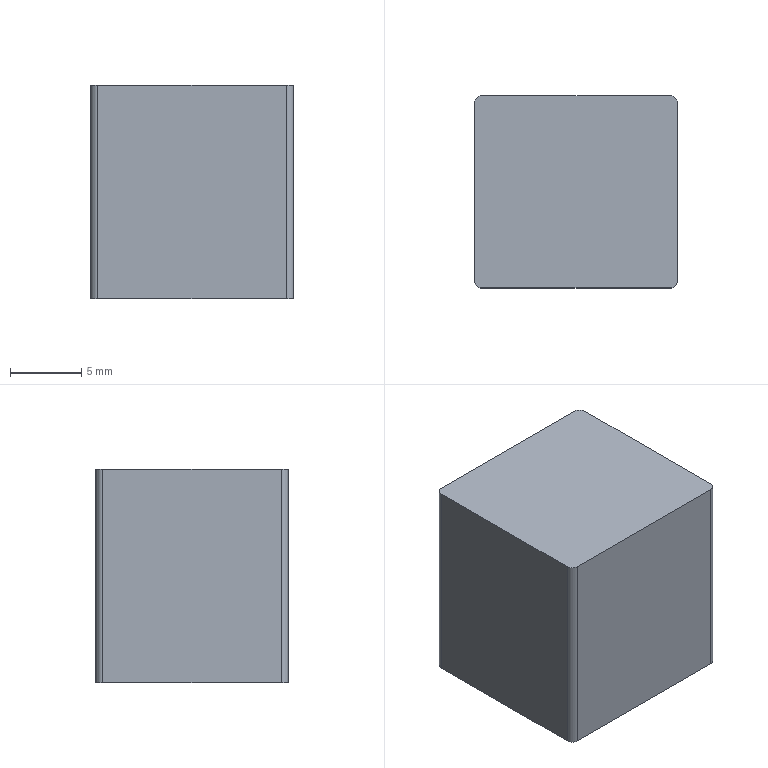Part | NX | features BREP 1 | 1 solid | 10 faces | box 14.274 x 13.522 x 15 mm | volume 2892 mm3 | plane 6 | cylinder 4 | commonest cylinder face diameters 1 x4
STEP:
#1=CARTESIAN_POINT('',(-6.637,6.761,-25.6));
#2=VERTEX_POINT('',#1);
#3=CARTESIAN_POINT('',(-7.137,6.261,-25.6));
#4=VERTEX_POINT('',#3);
#5=CARTESIAN_POINT('',(-6.637,6.261,-25.6));
#6=DIRECTION('',(0.,0.,1.));
#7=DIRECTION('',(1.,0.,0.));
#8=AXIS2_PLACEMENT_3D('',#5,#6,#7);
#9=CIRCLE('',#8,0.5);
#10=EDGE_CURVE('',#2,#4,#9,.T.);
#11=ORIENTED_EDGE('',*,*,#10,.F.);
#12=CARTESIAN_POINT('',(-6.637,6.761,-40.6));
#13=VERTEX_POINT('',#12);
#14=CARTESIAN_POINT('',(-6.637,6.761,-40.6));
#15=DIRECTION('',(0.,0.,1.));
#16=VECTOR('',#15,1000.);
#17=LINE('',#14,#16);
#18=EDGE_CURVE('',#13,#2,#17,.T.);
#19=ORIENTED_EDGE('',*,*,#18,.F.);
#20=CARTESIAN_POINT('',(-7.137,6.261,-40.6));
#21=VERTEX_POINT('',#20);
#22=CARTESIAN_POINT('',(-6.637,6.261,-40.6));
#23=DIRECTION('',(0.,0.,1.));
#24=DIRECTION('',(1.,0.,0.));
#25=AXIS2_PLACEMENT_3D('',#22,#23,#24);
#26=CIRCLE('',#25,0.5);
#27=EDGE_CURVE('',#13,#21,#26,.T.);
#28=ORIENTED_EDGE('',*,*,#27,.T.);
#29=CARTESIAN_POINT('',(-7.137,6.261,-40.6));
#30=DIRECTION('',(0.,0.,1.));
#31=VECTOR('',#30,1000.);
#32=LINE('',#29,#31);
#33=EDGE_CURVE('',#21,#4,#32,.T.);
#34=ORIENTED_EDGE('',*,*,#33,.T.);
#35=EDGE_LOOP('',(#11,#19,#28,#34));
#36=FACE_BOUND('',#35,.T.);
#37=CARTESIAN_POINT('',(-6.637,6.261,-40.6));
#38=DIRECTION('',(0.,0.,1.));
#39=DIRECTION('',(-1.,0.,0.));
#40=AXIS2_PLACEMENT_3D('',#37,#38,#39);
#41=CYLINDRICAL_SURFACE('',#40,0.5);
#42=ADVANCED_FACE('',(#36),#41,.T.);
#43=CARTESIAN_POINT('',(-7.137,-6.261,-25.6));
#44=VERTEX_POINT('',#43);
#45=CARTESIAN_POINT('',(-7.137,-6.261,-25.6));
#46=DIRECTION('',(0.,1.,0.));
#47=VECTOR('',#46,1000.);
#48=LINE('',#45,#47);
#49=EDGE_CURVE('',#44,#4,#48,.T.);
#50=ORIENTED_EDGE('',*,*,#49,.T.);
#51=ORIENTED_EDGE('',*,*,#33,.F.);
#52=CARTESIAN_POINT('',(-7.137,-6.261,-40.6));
#53=VERTEX_POINT('',#52);
#54=CARTESIAN_POINT('',(-7.137,-6.261,-40.6));
#55=DIRECTION('',(0.,1.,0.));
#56=VECTOR('',#55,1000.);
#57=LINE('',#54,#56);
#58=EDGE_CURVE('',#53,#21,#57,.T.);
#59=ORIENTED_EDGE('',*,*,#58,.F.);
#60=CARTESIAN_POINT('',(-7.137,-6.261,-40.6));
#61=DIRECTION('',(0.,0.,1.));
#62=VECTOR('',#61,1000.);
#63=LINE('',#60,#62);
#64=EDGE_CURVE('',#53,#44,#63,.T.);
#65=ORIENTED_EDGE('',*,*,#64,.T.);
#66=EDGE_LOOP('',(#50,#51,#59,#65));
#67=FACE_BOUND('',#66,.T.);
#68=CARTESIAN_POINT('',(-7.137,-6.261,-40.6));
#69=DIRECTION('',(1.,0.,0.));
#70=DIRECTION('',(0.,-1.,0.));
#71=AXIS2_PLACEMENT_3D('',#68,#69,#70);
#72=PLANE('',#71);
#73=ADVANCED_FACE('',(#67),#72,.F.);
#74=CARTESIAN_POINT('',(-6.637,-6.761,-25.6));
#75=VERTEX_POINT('',#74);
#76=CARTESIAN_POINT('',(-6.637,-6.261,-25.6));
#77=DIRECTION('',(0.,0.,1.));
#78=DIRECTION('',(1.,0.,0.));
#79=AXIS2_PLACEMENT_3D('',#76,#77,#78);
#80=CIRCLE('',#79,0.5);
#81=EDGE_CURVE('',#44,#75,#80,.T.);
#82=ORIENTED_EDGE('',*,*,#81,.F.);
#83=ORIENTED_EDGE('',*,*,#64,.F.);
#84=CARTESIAN_POINT('',(-6.637,-6.761,-40.6));
#85=VERTEX_POINT('',#84);
#86=CARTESIAN_POINT('',(-6.637,-6.261,-40.6));
#87=DIRECTION('',(0.,0.,1.));
#88=DIRECTION('',(1.,0.,0.));
#89=AXIS2_PLACEMENT_3D('',#86,#87,#88);
#90=CIRCLE('',#89,0.5);
#91=EDGE_CURVE('',#53,#85,#90,.T.);
#92=ORIENTED_EDGE('',*,*,#91,.T.);
#93=CARTESIAN_POINT('',(-6.637,-6.761,-40.6));
#94=DIRECTION('',(0.,0.,1.));
#95=VECTOR('',#94,1000.);
#96=LINE('',#93,#95);
#97=EDGE_CURVE('',#85,#75,#96,.T.);
#98=ORIENTED_EDGE('',*,*,#97,.T.);
#99=EDGE_LOOP('',(#82,#83,#92,#98));
#100=FACE_BOUND('',#99,.T.);
#101=CARTESIAN_POINT('',(-6.637,-6.261,-40.6));
#102=DIRECTION('',(0.,0.,1.));
#103=DIRECTION('',(-1.,0.,0.));
#104=AXIS2_PLACEMENT_3D('',#101,#102,#103);
#105=CYLINDRICAL_SURFACE('',#104,0.5);
#106=ADVANCED_FACE('',(#100),#105,.T.);
#107=CARTESIAN_POINT('',(6.637,-6.761,-25.6));
#108=VERTEX_POINT('',#107);
#109=CARTESIAN_POINT('',(6.637,-6.761,-25.6));
#110=DIRECTION('',(-1.,0.,0.));
#111=VECTOR('',#110,1000.);
#112=LINE('',#109,#111);
#113=EDGE_CURVE('',#108,#75,#112,.T.);
#114=ORIENTED_EDGE('',*,*,#113,.T.);
#115=ORIENTED_EDGE('',*,*,#97,.F.);
#116=CARTESIAN_POINT('',(6.637,-6.761,-40.6));
#117=VERTEX_POINT('',#116);
#118=CARTESIAN_POINT('',(6.637,-6.761,-40.6));
#119=DIRECTION('',(-1.,0.,0.));
#120=VECTOR('',#119,1000.);
#121=LINE('',#118,#120);
#122=EDGE_CURVE('',#117,#85,#121,.T.);
#123=ORIENTED_EDGE('',*,*,#122,.F.);
#124=CARTESIAN_POINT('',(6.637,-6.761,-40.6));
#125=DIRECTION('',(0.,0.,1.));
#126=VECTOR('',#125,1000.);
#127=LINE('',#124,#126);
#128=EDGE_CURVE('',#117,#108,#127,.T.);
#129=ORIENTED_EDGE('',*,*,#128,.T.);
#130=EDGE_LOOP('',(#114,#115,#123,#129));
#131=FACE_BOUND('',#130,.T.);
#132=CARTESIAN_POINT('',(6.637,-6.761,-40.6));
#133=DIRECTION('',(0.,1.,0.));
#134=DIRECTION('',(1.,0.,0.));
#135=AXIS2_PLACEMENT_3D('',#132,#133,#134);
#136=PLANE('',#135);
#137=ADVANCED_FACE('',(#131),#136,.F.);
#138=CARTESIAN_POINT('',(7.137,-6.261,-25.6));
#139=VERTEX_POINT('',#138);
#140=CARTESIAN_POINT('',(6.637,-6.261,-25.6));
#141=DIRECTION('',(0.,0.,1.));
#142=DIRECTION('',(1.,0.,0.));
#143=AXIS2_PLACEMENT_3D('',#140,#141,#142);
#144=CIRCLE('',#143,0.5);
#145=EDGE_CURVE('',#108,#139,#144,.T.);
#146=ORIENTED_EDGE('',*,*,#145,.F.);
#147=ORIENTED_EDGE('',*,*,#128,.F.);
#148=CARTESIAN_POINT('',(7.137,-6.261,-40.6));
#149=VERTEX_POINT('',#148);
#150=CARTESIAN_POINT('',(6.637,-6.261,-40.6));
#151=DIRECTION('',(0.,0.,1.));
#152=DIRECTION('',(1.,0.,0.));
#153=AXIS2_PLACEMENT_3D('',#150,#151,#152);
#154=CIRCLE('',#153,0.5);
#155=EDGE_CURVE('',#117,#149,#154,.T.);
#156=ORIENTED_EDGE('',*,*,#155,.T.);
#157=CARTESIAN_POINT('',(7.137,-6.261,-40.6));
#158=DIRECTION('',(0.,0.,1.));
#159=VECTOR('',#158,1000.);
#160=LINE('',#157,#159);
#161=EDGE_CURVE('',#149,#139,#160,.T.);
#162=ORIENTED_EDGE('',*,*,#161,.T.);
#163=EDGE_LOOP('',(#146,#147,#156,#162));
#164=FACE_BOUND('',#163,.T.);
#165=CARTESIAN_POINT('',(6.637,-6.261,-40.6));
#166=DIRECTION('',(0.,0.,1.));
#167=DIRECTION('',(-1.,0.,0.));
#168=AXIS2_PLACEMENT_3D('',#165,#166,#167);
#169=CYLINDRICAL_SURFACE('',#168,0.5);
#170=ADVANCED_FACE('',(#164),#169,.T.);
#171=CARTESIAN_POINT('',(7.137,6.261,-25.6));
#172=VERTEX_POINT('',#171);
#173=CARTESIAN_POINT('',(7.137,6.261,-25.6));
#174=DIRECTION('',(0.,-1.,0.));
#175=VECTOR('',#174,1000.);
#176=LINE('',#173,#175);
#177=EDGE_CURVE('',#172,#139,#176,.T.);
#178=ORIENTED_EDGE('',*,*,#177,.T.);
#179=ORIENTED_EDGE('',*,*,#161,.F.);
#180=CARTESIAN_POINT('',(7.137,6.261,-40.6));
#181=VERTEX_POINT('',#180);
#182=CARTESIAN_POINT('',(7.137,6.261,-40.6));
#183=DIRECTION('',(0.,-1.,0.));
#184=VECTOR('',#183,1000.);
#185=LINE('',#182,#184);
#186=EDGE_CURVE('',#181,#149,#185,.T.);
#187=ORIENTED_EDGE('',*,*,#186,.F.);
#188=CARTESIAN_POINT('',(7.137,6.261,-40.6));
#189=DIRECTION('',(0.,0.,1.));
#190=VECTOR('',#189,1000.);
#191=LINE('',#188,#190);
#192=EDGE_CURVE('',#181,#172,#191,.T.);
#193=ORIENTED_EDGE('',*,*,#192,.T.);
#194=EDGE_LOOP('',(#178,#179,#187,#193));
#195=FACE_BOUND('',#194,.T.);
#196=CARTESIAN_POINT('',(7.137,6.261,-40.6));
#197=DIRECTION('',(-1.,0.,0.));
#198=DIRECTION('',(0.,1.,0.));
#199=AXIS2_PLACEMENT_3D('',#196,#197,#198);
#200=PLANE('',#199);
#201=ADVANCED_FACE('',(#195),#200,.F.);
#202=CARTESIAN_POINT('',(6.637,6.761,-25.6));
#203=VERTEX_POINT('',#202);
#204=CARTESIAN_POINT('',(6.637,6.261,-25.6));
#205=DIRECTION('',(0.,0.,1.));
#206=DIRECTION('',(1.,0.,0.));
#207=AXIS2_PLACEMENT_3D('',#204,#205,#206);
#208=CIRCLE('',#207,0.5);
#209=EDGE_CURVE('',#172,#203,#208,.T.);
#210=ORIENTED_EDGE('',*,*,#209,.F.);
#211=ORIENTED_EDGE('',*,*,#192,.F.);
#212=CARTESIAN_POINT('',(6.637,6.761,-40.6));
#213=VERTEX_POINT('',#212);
#214=CARTESIAN_POINT('',(6.637,6.261,-40.6));
#215=DIRECTION('',(0.,0.,1.));
#216=DIRECTION('',(1.,0.,0.));
#217=AXIS2_PLACEMENT_3D('',#214,#215,#216);
#218=CIRCLE('',#217,0.5);
#219=EDGE_CURVE('',#181,#213,#218,.T.);
#220=ORIENTED_EDGE('',*,*,#219,.T.);
#221=CARTESIAN_POINT('',(6.637,6.761,-40.6));
#222=DIRECTION('',(0.,0.,1.));
#223=VECTOR('',#222,1000.);
#224=LINE('',#221,#223);
#225=EDGE_CURVE('',#213,#203,#224,.T.);
#226=ORIENTED_EDGE('',*,*,#225,.T.);
#227=EDGE_LOOP('',(#210,#211,#220,#226));
#228=FACE_BOUND('',#227,.T.);
#229=CARTESIAN_POINT('',(6.637,6.261,-40.6));
#230=DIRECTION('',(0.,0.,1.));
#231=DIRECTION('',(-1.,0.,0.));
#232=AXIS2_PLACEMENT_3D('',#229,#230,#231);
#233=CYLINDRICAL_SURFACE('',#232,0.5);
#234=ADVANCED_FACE('',(#228),#233,.T.);
#235=CARTESIAN_POINT('',(-6.637,6.761,-25.6));
#236=DIRECTION('',(1.,0.,0.));
#237=VECTOR('',#236,1000.);
#238=LINE('',#235,#237);
#239=EDGE_CURVE('',#2,#203,#238,.T.);
#240=ORIENTED_EDGE('',*,*,#239,.T.);
#241=ORIENTED_EDGE('',*,*,#225,.F.);
#242=CARTESIAN_POINT('',(-6.637,6.761,-40.6));
#243=DIRECTION('',(1.,0.,0.));
#244=VECTOR('',#243,1000.);
#245=LINE('',#242,#244);
#246=EDGE_CURVE('',#13,#213,#245,.T.);
#247=ORIENTED_EDGE('',*,*,#246,.F.);
#248=ORIENTED_EDGE('',*,*,#18,.T.);
#249=EDGE_LOOP('',(#240,#241,#247,#248));
#250=FACE_BOUND('',#249,.T.);
#251=CARTESIAN_POINT('',(-6.637,6.761,-40.6));
#252=DIRECTION('',(0.,-1.,0.));
#253=DIRECTION('',(0.,0.,1.));
#254=AXIS2_PLACEMENT_3D('',#251,#252,#253);
#255=PLANE('',#254);
#256=ADVANCED_FACE('',(#250),#255,.F.);
#257=ORIENTED_EDGE('',*,*,#27,.F.);
#258=ORIENTED_EDGE('',*,*,#246,.T.);
#259=ORIENTED_EDGE('',*,*,#219,.F.);
#260=ORIENTED_EDGE('',*,*,#186,.T.);
#261=ORIENTED_EDGE('',*,*,#155,.F.);
#262=ORIENTED_EDGE('',*,*,#122,.T.);
#263=ORIENTED_EDGE('',*,*,#91,.F.);
#264=ORIENTED_EDGE('',*,*,#58,.T.);
#265=EDGE_LOOP('',(#257,#258,#259,#260,#261,#262,#263,#264));
#266=FACE_BOUND('',#265,.T.);
#267=CARTESIAN_POINT('',(-6.637,6.261,-40.6));
#268=DIRECTION('',(0.,0.,1.));
#269=DIRECTION('',(-1.,0.,0.));
#270=AXIS2_PLACEMENT_3D('',#267,#268,#269);
#271=PLANE('',#270);
#272=ADVANCED_FACE('',(#266),#271,.F.);
#273=ORIENTED_EDGE('',*,*,#10,.T.);
#274=ORIENTED_EDGE('',*,*,#49,.F.);
#275=ORIENTED_EDGE('',*,*,#81,.T.);
#276=ORIENTED_EDGE('',*,*,#113,.F.);
#277=ORIENTED_EDGE('',*,*,#145,.T.);
#278=ORIENTED_EDGE('',*,*,#177,.F.);
#279=ORIENTED_EDGE('',*,*,#209,.T.);
#280=ORIENTED_EDGE('',*,*,#239,.F.);
#281=EDGE_LOOP('',(#273,#274,#275,#276,#277,#278,#279,#280));
#282=FACE_BOUND('',#281,.T.);
#283=CARTESIAN_POINT('',(-6.637,6.261,-25.6));
#284=DIRECTION('',(0.,0.,1.));
#285=DIRECTION('',(-1.,0.,0.));
#286=AXIS2_PLACEMENT_3D('',#283,#284,#285);
#287=PLANE('',#286);
#288=ADVANCED_FACE('',(#282),#287,.T.);
#289=CLOSED_SHELL('',(#42,#73,#106,#137,#170,#201,#234,#256,#272,#288));
#290=MANIFOLD_SOLID_BREP('',#289);
#291=(LENGTH_UNIT()NAMED_UNIT(*)SI_UNIT(.MILLI.,.METRE.));
#292=UNCERTAINTY_MEASURE_WITH_UNIT(LENGTH_MEASURE(0.00001),#291,'','');
#293=(NAMED_UNIT(*)PLANE_ANGLE_UNIT()SI_UNIT($,.RADIAN.));
#294=(NAMED_UNIT(*)SI_UNIT($,.STERADIAN.)SOLID_ANGLE_UNIT());
#295=(GEOMETRIC_REPRESENTATION_CONTEXT(3)GLOBAL_UNCERTAINTY_ASSIGNED_CONTEXT((#292))GLOBAL_UNIT_ASSIGNED_CONTEXT((#291,#293,#294))REPRESENTATION_CONTEXT('',''));
#296=ADVANCED_BREP_SHAPE_REPRESENTATION('',(#290),#295);